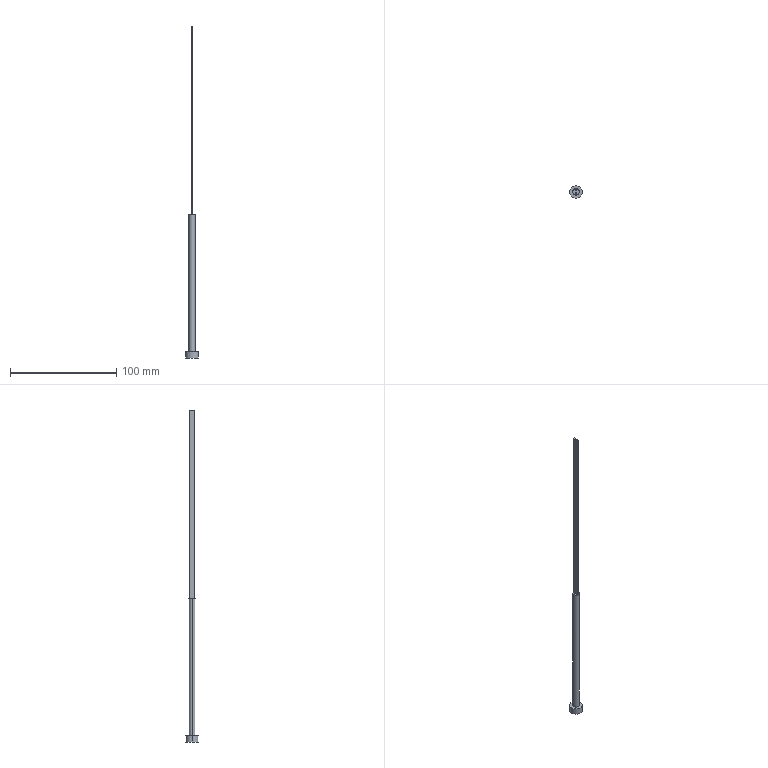Part | Creo | 1 solid | 12 faces | box 12 x 12 x 312.599 mm | volume 5498 mm3 | plane 8 | cylinder 4 | commonest cylinder face diameters 6 x2 12 x2
STEP:
#1=CARTESIAN_POINT('',(-105.609,-81.1,52.099));
#2=VERTEX_POINT('',#1);
#3=CARTESIAN_POINT('',(-105.609,-81.1,-125.5));
#4=VERTEX_POINT('',#3);
#5=CARTESIAN_POINT('',(-105.609,-81.1,52.099));
#6=DIRECTION('',(0.,0.,-1.));
#7=VECTOR('',#6,177.599);
#8=LINE('',#5,#7);
#9=EDGE_CURVE('',#2,#4,#8,.T.);
#10=ORIENTED_EDGE('',*,*,#9,.F.);
#11=CARTESIAN_POINT('',(-105.609,-86.6,52.099));
#12=VERTEX_POINT('',#11);
#13=CARTESIAN_POINT('',(-105.609,-81.1,52.099));
#14=DIRECTION('',(0.,-1.,0.));
#15=VECTOR('',#14,5.5);
#16=LINE('',#13,#15);
#17=EDGE_CURVE('',#2,#12,#16,.T.);
#18=ORIENTED_EDGE('',*,*,#17,.T.);
#19=CARTESIAN_POINT('',(-105.609,-86.6,-125.5));
#20=VERTEX_POINT('',#19);
#21=CARTESIAN_POINT('',(-105.609,-86.6,52.099));
#22=DIRECTION('',(0.,0.,-1.));
#23=VECTOR('',#22,177.599);
#24=LINE('',#21,#23);
#25=EDGE_CURVE('',#12,#20,#24,.T.);
#26=ORIENTED_EDGE('',*,*,#25,.T.);
#27=CARTESIAN_POINT('',(-105.609,-86.6,-125.5));
#28=DIRECTION('',(0.,1.,0.));
#29=VECTOR('',#28,5.5);
#30=LINE('',#27,#29);
#31=EDGE_CURVE('',#20,#4,#30,.T.);
#32=ORIENTED_EDGE('',*,*,#31,.T.);
#33=EDGE_LOOP('',(#10,#18,#26,#32));
#34=FACE_OUTER_BOUND('',#33,.F.);
#35=CARTESIAN_POINT('',(-105.609,-86.6,-77.901));
#36=DIRECTION('',(1.,0.,0.));
#37=DIRECTION('',(0.,1.,0.));
#38=AXIS2_PLACEMENT_3D('',#35,#36,#37);
#39=PLANE('',#38);
#40=ADVANCED_FACE('',(#34),#39,.F.);
#41=CARTESIAN_POINT('',(-104.409,-81.1,52.099));
#42=VERTEX_POINT('',#41);
#43=CARTESIAN_POINT('',(-104.409,-81.1,-125.5));
#44=VERTEX_POINT('',#43);
#45=CARTESIAN_POINT('',(-104.409,-81.1,52.099));
#46=DIRECTION('',(0.,0.,-1.));
#47=VECTOR('',#46,177.599);
#48=LINE('',#45,#47);
#49=EDGE_CURVE('',#42,#44,#48,.T.);
#50=ORIENTED_EDGE('',*,*,#49,.F.);
#51=CARTESIAN_POINT('',(-104.409,-81.1,52.099));
#52=DIRECTION('',(-1.,0.,0.));
#53=VECTOR('',#52,1.2);
#54=LINE('',#51,#53);
#55=EDGE_CURVE('',#42,#2,#54,.T.);
#56=ORIENTED_EDGE('',*,*,#55,.T.);
#57=ORIENTED_EDGE('',*,*,#9,.T.);
#58=CARTESIAN_POINT('',(-105.609,-81.1,-125.5));
#59=DIRECTION('',(1.,0.,0.));
#60=VECTOR('',#59,1.2);
#61=LINE('',#58,#60);
#62=EDGE_CURVE('',#4,#44,#61,.T.);
#63=ORIENTED_EDGE('',*,*,#62,.T.);
#64=EDGE_LOOP('',(#50,#56,#57,#63));
#65=FACE_OUTER_BOUND('',#64,.F.);
#66=CARTESIAN_POINT('',(-105.609,-81.1,-77.901));
#67=DIRECTION('',(0.,-1.,0.));
#68=DIRECTION('',(1.,0.,0.));
#69=AXIS2_PLACEMENT_3D('',#66,#67,#68);
#70=PLANE('',#69);
#71=ADVANCED_FACE('',(#65),#70,.F.);
#72=CARTESIAN_POINT('',(-104.409,-86.6,52.099));
#73=VERTEX_POINT('',#72);
#74=CARTESIAN_POINT('',(-104.409,-86.6,-125.5));
#75=VERTEX_POINT('',#74);
#76=CARTESIAN_POINT('',(-104.409,-86.6,52.099));
#77=DIRECTION('',(0.,0.,-1.));
#78=VECTOR('',#77,177.599);
#79=LINE('',#76,#78);
#80=EDGE_CURVE('',#73,#75,#79,.T.);
#81=ORIENTED_EDGE('',*,*,#80,.F.);
#82=CARTESIAN_POINT('',(-104.409,-86.6,52.099));
#83=DIRECTION('',(0.,1.,0.));
#84=VECTOR('',#83,5.5);
#85=LINE('',#82,#84);
#86=EDGE_CURVE('',#73,#42,#85,.T.);
#87=ORIENTED_EDGE('',*,*,#86,.T.);
#88=ORIENTED_EDGE('',*,*,#49,.T.);
#89=CARTESIAN_POINT('',(-104.409,-81.1,-125.5));
#90=DIRECTION('',(0.,-1.,0.));
#91=VECTOR('',#90,5.5);
#92=LINE('',#89,#91);
#93=EDGE_CURVE('',#44,#75,#92,.T.);
#94=ORIENTED_EDGE('',*,*,#93,.T.);
#95=EDGE_LOOP('',(#81,#87,#88,#94));
#96=FACE_OUTER_BOUND('',#95,.F.);
#97=CARTESIAN_POINT('',(-104.409,-81.1,-77.901));
#98=DIRECTION('',(-1.,0.,0.));
#99=DIRECTION('',(0.,-1.,0.));
#100=AXIS2_PLACEMENT_3D('',#97,#98,#99);
#101=PLANE('',#100);
#102=ADVANCED_FACE('',(#96),#101,.F.);
#103=ORIENTED_EDGE('',*,*,#25,.F.);
#104=CARTESIAN_POINT('',(-105.609,-86.6,52.099));
#105=DIRECTION('',(1.,0.,0.));
#106=VECTOR('',#105,1.2);
#107=LINE('',#104,#106);
#108=EDGE_CURVE('',#12,#73,#107,.T.);
#109=ORIENTED_EDGE('',*,*,#108,.T.);
#110=ORIENTED_EDGE('',*,*,#80,.T.);
#111=CARTESIAN_POINT('',(-104.409,-86.6,-125.5));
#112=DIRECTION('',(-1.,0.,0.));
#113=VECTOR('',#112,1.2);
#114=LINE('',#111,#113);
#115=EDGE_CURVE('',#75,#20,#114,.T.);
#116=ORIENTED_EDGE('',*,*,#115,.T.);
#117=EDGE_LOOP('',(#103,#109,#110,#116));
#118=FACE_OUTER_BOUND('',#117,.F.);
#119=CARTESIAN_POINT('',(-104.409,-86.6,-77.901));
#120=DIRECTION('',(0.,1.,0.));
#121=DIRECTION('',(-1.,0.,0.));
#122=AXIS2_PLACEMENT_3D('',#119,#120,#121);
#123=PLANE('',#122);
#124=ADVANCED_FACE('',(#118),#123,.F.);
#125=ORIENTED_EDGE('',*,*,#17,.F.);
#126=ORIENTED_EDGE('',*,*,#55,.F.);
#127=ORIENTED_EDGE('',*,*,#86,.F.);
#128=ORIENTED_EDGE('',*,*,#108,.F.);
#129=EDGE_LOOP('',(#125,#126,#127,#128));
#130=FACE_OUTER_BOUND('',#129,.F.);
#131=CARTESIAN_POINT('',(-105.609,-81.1,52.099));
#132=DIRECTION('',(0.,0.,-1.));
#133=DIRECTION('',(-1.,0.,0.));
#134=AXIS2_PLACEMENT_3D('',#131,#132,#133);
#135=PLANE('',#134);
#136=ADVANCED_FACE('',(#130),#135,.F.);
#137=CARTESIAN_POINT('',(-102.009,-83.85,-125.5));
#138=VERTEX_POINT('',#137);
#139=CARTESIAN_POINT('',(-108.009,-83.85,-125.5));
#140=VERTEX_POINT('',#139);
#141=CARTESIAN_POINT('',(-105.009,-83.85,-125.5));
#142=DIRECTION('',(0.,0.,1.));
#143=DIRECTION('',(1.,0.,0.));
#144=AXIS2_PLACEMENT_3D('',#141,#142,#143);
#145=CIRCLE('',#144,3.);
#146=EDGE_CURVE('',#138,#140,#145,.T.);
#147=ORIENTED_EDGE('',*,*,#146,.F.);
#148=CARTESIAN_POINT('',(-105.009,-83.85,-125.5));
#149=DIRECTION('',(0.,0.,1.));
#150=DIRECTION('',(-1.,0.,0.));
#151=AXIS2_PLACEMENT_3D('',#148,#149,#150);
#152=CIRCLE('',#151,3.);
#153=EDGE_CURVE('',#140,#138,#152,.T.);
#154=ORIENTED_EDGE('',*,*,#153,.F.);
#155=EDGE_LOOP('',(#147,#154));
#156=FACE_OUTER_BOUND('',#155,.F.);
#157=ORIENTED_EDGE('',*,*,#31,.F.);
#158=ORIENTED_EDGE('',*,*,#115,.F.);
#159=ORIENTED_EDGE('',*,*,#93,.F.);
#160=ORIENTED_EDGE('',*,*,#62,.F.);
#161=EDGE_LOOP('',(#157,#158,#159,#160));
#162=FACE_BOUND('',#161,.F.);
#163=CARTESIAN_POINT('',(-105.009,-83.85,-125.5));
#164=DIRECTION('',(0.,0.,1.));
#165=DIRECTION('',(1.,0.,0.));
#166=AXIS2_PLACEMENT_3D('',#163,#164,#165);
#167=PLANE('',#166);
#168=ADVANCED_FACE('',(#156,#162),#167,.T.);
#169=CARTESIAN_POINT('',(-108.009,-83.85,-254.5));
#170=VERTEX_POINT('',#169);
#171=CARTESIAN_POINT('',(-102.009,-83.85,-254.5));
#172=VERTEX_POINT('',#171);
#173=CARTESIAN_POINT('',(-105.009,-83.85,-254.5));
#174=DIRECTION('',(0.,0.,-1.));
#175=DIRECTION('',(-1.,0.,0.));
#176=AXIS2_PLACEMENT_3D('',#173,#174,#175);
#177=CIRCLE('',#176,3.);
#178=EDGE_CURVE('',#170,#172,#177,.T.);
#179=ORIENTED_EDGE('',*,*,#178,.T.);
#180=CARTESIAN_POINT('',(-102.009,-83.85,-254.5));
#181=DIRECTION('',(0.,0.,1.));
#182=VECTOR('',#181,129.);
#183=LINE('',#180,#182);
#184=EDGE_CURVE('',#172,#138,#183,.T.);
#185=ORIENTED_EDGE('',*,*,#184,.T.);
#186=ORIENTED_EDGE('',*,*,#146,.T.);
#187=CARTESIAN_POINT('',(-108.009,-83.85,-254.5));
#188=DIRECTION('',(0.,0.,1.));
#189=VECTOR('',#188,129.);
#190=LINE('',#187,#189);
#191=EDGE_CURVE('',#170,#140,#190,.T.);
#192=ORIENTED_EDGE('',*,*,#191,.F.);
#193=EDGE_LOOP('',(#179,#185,#186,#192));
#194=FACE_OUTER_BOUND('',#193,.F.);
#195=CARTESIAN_POINT('',(-105.009,-83.85,-260.5));
#196=DIRECTION('',(0.,0.,1.));
#197=DIRECTION('',(1.,0.,0.));
#198=AXIS2_PLACEMENT_3D('',#195,#196,#197);
#199=CYLINDRICAL_SURFACE('',#198,3.);
#200=ADVANCED_FACE('',(#194),#199,.T.);
#201=CARTESIAN_POINT('',(-99.009,-83.85,-254.5));
#202=VERTEX_POINT('',#201);
#203=CARTESIAN_POINT('',(-111.009,-83.85,-254.5));
#204=VERTEX_POINT('',#203);
#205=CARTESIAN_POINT('',(-105.009,-83.85,-254.5));
#206=DIRECTION('',(0.,0.,1.));
#207=DIRECTION('',(1.,0.,0.));
#208=AXIS2_PLACEMENT_3D('',#205,#206,#207);
#209=CIRCLE('',#208,6.);
#210=EDGE_CURVE('',#202,#204,#209,.T.);
#211=ORIENTED_EDGE('',*,*,#210,.F.);
#212=CARTESIAN_POINT('',(-105.009,-83.85,-254.5));
#213=DIRECTION('',(0.,0.,1.));
#214=DIRECTION('',(-1.,0.,0.));
#215=AXIS2_PLACEMENT_3D('',#212,#213,#214);
#216=CIRCLE('',#215,6.);
#217=EDGE_CURVE('',#204,#202,#216,.T.);
#218=ORIENTED_EDGE('',*,*,#217,.F.);
#219=EDGE_LOOP('',(#211,#218));
#220=FACE_OUTER_BOUND('',#219,.F.);
#221=CARTESIAN_POINT('',(-105.009,-83.85,-254.5));
#222=DIRECTION('',(0.,0.,-1.));
#223=DIRECTION('',(1.,0.,0.));
#224=AXIS2_PLACEMENT_3D('',#221,#222,#223);
#225=CIRCLE('',#224,3.);
#226=EDGE_CURVE('',#172,#170,#225,.T.);
#227=ORIENTED_EDGE('',*,*,#226,.F.);
#228=ORIENTED_EDGE('',*,*,#178,.F.);
#229=EDGE_LOOP('',(#227,#228));
#230=FACE_BOUND('',#229,.F.);
#231=CARTESIAN_POINT('',(-105.009,-83.85,-254.5));
#232=DIRECTION('',(0.,0.,1.));
#233=DIRECTION('',(1.,0.,0.));
#234=AXIS2_PLACEMENT_3D('',#231,#232,#233);
#235=PLANE('',#234);
#236=ADVANCED_FACE('',(#220,#230),#235,.T.);
#237=ORIENTED_EDGE('',*,*,#226,.T.);
#238=ORIENTED_EDGE('',*,*,#191,.T.);
#239=ORIENTED_EDGE('',*,*,#153,.T.);
#240=ORIENTED_EDGE('',*,*,#184,.F.);
#241=EDGE_LOOP('',(#237,#238,#239,#240));
#242=FACE_OUTER_BOUND('',#241,.F.);
#243=CARTESIAN_POINT('',(-105.009,-83.85,-260.5));
#244=DIRECTION('',(0.,0.,1.));
#245=DIRECTION('',(1.,0.,0.));
#246=AXIS2_PLACEMENT_3D('',#243,#244,#245);
#247=CYLINDRICAL_SURFACE('',#246,3.);
#248=ADVANCED_FACE('',(#242),#247,.T.);
#249=ORIENTED_EDGE('',*,*,#210,.T.);
#250=CARTESIAN_POINT('',(-111.009,-83.85,-260.5));
#251=VERTEX_POINT('',#250);
#252=CARTESIAN_POINT('',(-111.009,-83.85,-260.5));
#253=DIRECTION('',(0.,0.,1.));
#254=VECTOR('',#253,6.);
#255=LINE('',#252,#254);
#256=EDGE_CURVE('',#251,#204,#255,.T.);
#257=ORIENTED_EDGE('',*,*,#256,.F.);
#258=CARTESIAN_POINT('',(-99.009,-83.85,-260.5));
#259=VERTEX_POINT('',#258);
#260=CARTESIAN_POINT('',(-105.009,-83.85,-260.5));
#261=DIRECTION('',(0.,0.,-1.));
#262=DIRECTION('',(-1.,0.,0.));
#263=AXIS2_PLACEMENT_3D('',#260,#261,#262);
#264=CIRCLE('',#263,6.);
#265=EDGE_CURVE('',#251,#259,#264,.T.);
#266=ORIENTED_EDGE('',*,*,#265,.T.);
#267=CARTESIAN_POINT('',(-99.009,-83.85,-260.5));
#268=DIRECTION('',(0.,0.,1.));
#269=VECTOR('',#268,6.);
#270=LINE('',#267,#269);
#271=EDGE_CURVE('',#259,#202,#270,.T.);
#272=ORIENTED_EDGE('',*,*,#271,.T.);
#273=EDGE_LOOP('',(#249,#257,#266,#272));
#274=FACE_OUTER_BOUND('',#273,.F.);
#275=CARTESIAN_POINT('',(-105.009,-83.85,-260.5));
#276=DIRECTION('',(0.,0.,1.));
#277=DIRECTION('',(1.,0.,0.));
#278=AXIS2_PLACEMENT_3D('',#275,#276,#277);
#279=CYLINDRICAL_SURFACE('',#278,6.);
#280=ADVANCED_FACE('',(#274),#279,.T.);
#281=ORIENTED_EDGE('',*,*,#217,.T.);
#282=ORIENTED_EDGE('',*,*,#271,.F.);
#283=CARTESIAN_POINT('',(-105.009,-83.85,-260.5));
#284=DIRECTION('',(0.,0.,-1.));
#285=DIRECTION('',(1.,0.,0.));
#286=AXIS2_PLACEMENT_3D('',#283,#284,#285);
#287=CIRCLE('',#286,6.);
#288=EDGE_CURVE('',#259,#251,#287,.T.);
#289=ORIENTED_EDGE('',*,*,#288,.T.);
#290=ORIENTED_EDGE('',*,*,#256,.T.);
#291=EDGE_LOOP('',(#281,#282,#289,#290));
#292=FACE_OUTER_BOUND('',#291,.F.);
#293=CARTESIAN_POINT('',(-105.009,-83.85,-260.5));
#294=DIRECTION('',(0.,0.,1.));
#295=DIRECTION('',(1.,0.,0.));
#296=AXIS2_PLACEMENT_3D('',#293,#294,#295);
#297=CYLINDRICAL_SURFACE('',#296,6.);
#298=ADVANCED_FACE('',(#292),#297,.T.);
#299=ORIENTED_EDGE('',*,*,#288,.F.);
#300=ORIENTED_EDGE('',*,*,#265,.F.);
#301=EDGE_LOOP('',(#299,#300));
#302=FACE_OUTER_BOUND('',#301,.F.);
#303=CARTESIAN_POINT('',(143.614,83.015,-260.5));
#304=DIRECTION('',(0.,0.,-1.));
#305=DIRECTION('',(1.,0.,0.));
#306=AXIS2_PLACEMENT_3D('',#303,#304,#305);
#307=PLANE('',#306);
#308=ADVANCED_FACE('',(#302),#307,.T.);
#309=CLOSED_SHELL('',(#40,#71,#102,#124,#136,#168,#200,#236,#248,#280,#298,#308));
#310=MANIFOLD_SOLID_BREP('',#309);
#311=(LENGTH_UNIT()NAMED_UNIT(*)SI_UNIT(.MILLI.,.METRE.));
#312=UNCERTAINTY_MEASURE_WITH_UNIT(LENGTH_MEASURE(0.0313),#311,'','');
#313=(NAMED_UNIT(*)PLANE_ANGLE_UNIT()SI_UNIT($,.RADIAN.));
#314=PLANE_ANGLE_MEASURE_WITH_UNIT(PLANE_ANGLE_MEASURE(0.01745),#313);
#315=(CONVERSION_BASED_UNIT('DEGREE',#314)NAMED_UNIT(*)PLANE_ANGLE_UNIT());
#316=(NAMED_UNIT(*)SI_UNIT($,.STERADIAN.)SOLID_ANGLE_UNIT());
#317=(GEOMETRIC_REPRESENTATION_CONTEXT(3)GLOBAL_UNCERTAINTY_ASSIGNED_CONTEXT((#312))GLOBAL_UNIT_ASSIGNED_CONTEXT((#311,#315,#316))REPRESENTATION_CONTEXT('',''));
#318=ADVANCED_BREP_SHAPE_REPRESENTATION('',(#310),#317);